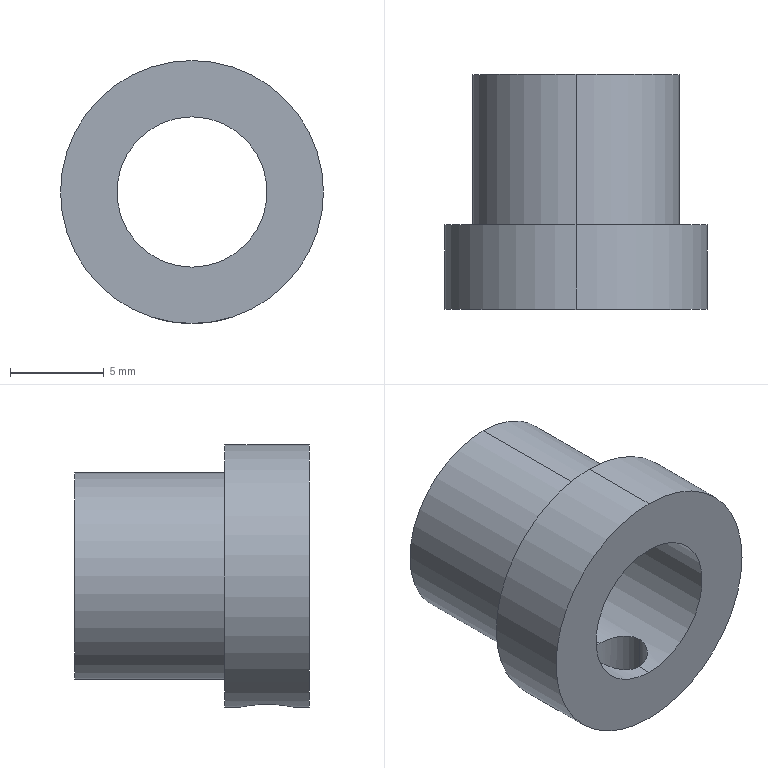Part | SolidWorks | features ICE 1, Revolution 1 | 1 solid | 11 faces | box 14 x 12.5 x 14 mm | volume 803.242 mm3 | cylinder 8 | plane 3 | commonest cylinder face diameters 3 x2 8 x2 11 x2 14 x2
STEP:
#1=CARTESIAN_POINT('',(0.,-4.489,-7.));
#2=VERTEX_POINT('',#1);
#3=CARTESIAN_POINT('',(-1.5,-2.989,-6.837));
#4=VERTEX_POINT('',#3);
#5=CARTESIAN_POINT('',(0.,-4.489,-7.));
#6=CARTESIAN_POINT('',(-0.1961,-4.489,-7.));
#7=CARTESIAN_POINT('',(-0.3941,-4.449,-6.991));
#8=CARTESIAN_POINT('',(-0.7554,-4.299,-6.961));
#9=CARTESIAN_POINT('',(-0.922,-4.188,-6.94));
#10=CARTESIAN_POINT('',(-1.13,-3.98,-6.909));
#11=CARTESIAN_POINT('',(-1.193,-3.904,-6.898));
#12=CARTESIAN_POINT('',(-1.301,-3.741,-6.878));
#13=CARTESIAN_POINT('',(-1.347,-3.655,-6.869));
#14=CARTESIAN_POINT('',(-1.461,-3.382,-6.846));
#15=CARTESIAN_POINT('',(-1.5,-3.187,-6.837));
#16=CARTESIAN_POINT('',(-1.5,-2.989,-6.837));
#17=B_SPLINE_CURVE_WITH_KNOTS('',3,(#5,#6,#7,#8,#9,#10,#11,#12,#13,#14,#15,#16),.UNSPECIFIED.,.F.,.F.,(4,2,2,2,2,4),(0.004703,0.005291,0.005879,0.006173,0.006467,0.007055),.UNSPECIFIED.);
#18=EDGE_CURVE('',#2,#4,#17,.T.);
#19=ORIENTED_EDGE('',*,*,#18,.T.);
#20=CARTESIAN_POINT('',(-1.5,-2.989,-3.708));
#21=VERTEX_POINT('',#20);
#22=CARTESIAN_POINT('',(-1.5,-2.989,-10.));
#23=DIRECTION('',(0.,0.,1.));
#24=VECTOR('',#23,1000.);
#25=LINE('',#22,#24);
#26=EDGE_CURVE('',#4,#21,#25,.T.);
#27=ORIENTED_EDGE('',*,*,#26,.T.);
#28=CARTESIAN_POINT('',(0.,-4.489,-4.));
#29=VERTEX_POINT('',#28);
#30=CARTESIAN_POINT('',(-1.5,-2.989,-3.708));
#31=CARTESIAN_POINT('',(-1.5,-3.087,-3.708));
#32=CARTESIAN_POINT('',(-1.49,-3.188,-3.712));
#33=CARTESIAN_POINT('',(-1.451,-3.381,-3.728));
#34=CARTESIAN_POINT('',(-1.422,-3.475,-3.739));
#35=CARTESIAN_POINT('',(-1.346,-3.658,-3.767));
#36=CARTESIAN_POINT('',(-1.3,-3.744,-3.783));
#37=CARTESIAN_POINT('',(-1.192,-3.905,-3.819));
#38=CARTESIAN_POINT('',(-1.129,-3.981,-3.838));
#39=CARTESIAN_POINT('',(-0.9911,-4.119,-3.876));
#40=CARTESIAN_POINT('',(-0.9163,-4.18,-3.895));
#41=CARTESIAN_POINT('',(-0.7543,-4.289,-3.929));
#42=CARTESIAN_POINT('',(-0.6667,-4.336,-3.945));
#43=CARTESIAN_POINT('',(-0.3961,-4.449,-3.985));
#44=CARTESIAN_POINT('',(-0.1971,-4.489,-4.));
#45=CARTESIAN_POINT('',(0.,-4.489,-4.));
#46=B_SPLINE_CURVE_WITH_KNOTS('',3,(#30,#31,#32,#33,#34,#35,#36,#37,#38,#39,#40,#41,#42,#43,#44,#45),.UNSPECIFIED.,.F.,.F.,(4,2,2,2,2,2,2,4),(0.002368,0.002663,0.002959,0.003255,0.00355,0.003846,0.004142,0.004733),.UNSPECIFIED.);
#47=EDGE_CURVE('',#21,#29,#46,.T.);
#48=ORIENTED_EDGE('',*,*,#47,.T.);
#49=CARTESIAN_POINT('',(1.5,-2.989,-3.708));
#50=VERTEX_POINT('',#49);
#51=CARTESIAN_POINT('',(0.,-4.489,-4.));
#52=CARTESIAN_POINT('',(0.1971,-4.489,-4.));
#53=CARTESIAN_POINT('',(0.3959,-4.449,-3.985));
#54=CARTESIAN_POINT('',(0.6677,-4.335,-3.945));
#55=CARTESIAN_POINT('',(0.7553,-4.288,-3.929));
#56=CARTESIAN_POINT('',(0.9168,-4.18,-3.894));
#57=CARTESIAN_POINT('',(0.9919,-4.118,-3.876));
#58=CARTESIAN_POINT('',(1.2,-3.91,-3.819));
#59=CARTESIAN_POINT('',(1.309,-3.747,-3.781));
#60=CARTESIAN_POINT('',(1.423,-3.474,-3.739));
#61=CARTESIAN_POINT('',(1.451,-3.381,-3.728));
#62=CARTESIAN_POINT('',(1.49,-3.188,-3.712));
#63=CARTESIAN_POINT('',(1.5,-3.087,-3.708));
#64=CARTESIAN_POINT('',(1.5,-2.989,-3.708));
#65=B_SPLINE_CURVE_WITH_KNOTS('',3,(#51,#52,#53,#54,#55,#56,#57,#58,#59,#60,#61,#62,#63,#64),.UNSPECIFIED.,.F.,.F.,(4,2,2,2,2,2,4),(0.004733,0.005325,0.00562,0.005916,0.006508,0.006803,0.007099),.UNSPECIFIED.);
#66=EDGE_CURVE('',#29,#50,#65,.T.);
#67=ORIENTED_EDGE('',*,*,#66,.T.);
#68=CARTESIAN_POINT('',(1.5,-2.989,-6.837));
#69=VERTEX_POINT('',#68);
#70=CARTESIAN_POINT('',(1.5,-2.989,-10.));
#71=DIRECTION('',(0.,0.,1.));
#72=VECTOR('',#71,1000.);
#73=LINE('',#70,#72);
#74=EDGE_CURVE('',#69,#50,#73,.T.);
#75=ORIENTED_EDGE('',*,*,#74,.F.);
#76=CARTESIAN_POINT('',(1.5,-2.989,-6.837));
#77=CARTESIAN_POINT('',(1.5,-3.087,-6.837));
#78=CARTESIAN_POINT('',(1.49,-3.186,-6.84));
#79=CARTESIAN_POINT('',(1.452,-3.379,-6.848));
#80=CARTESIAN_POINT('',(1.423,-3.473,-6.854));
#81=CARTESIAN_POINT('',(1.31,-3.745,-6.877));
#82=CARTESIAN_POINT('',(1.2,-3.91,-6.898));
#83=CARTESIAN_POINT('',(0.9907,-4.119,-6.93));
#84=CARTESIAN_POINT('',(0.9152,-4.181,-6.94));
#85=CARTESIAN_POINT('',(0.753,-4.29,-6.96));
#86=CARTESIAN_POINT('',(0.6652,-4.337,-6.969));
#87=CARTESIAN_POINT('',(0.484,-4.412,-6.984));
#88=CARTESIAN_POINT('',(0.3905,-4.44,-6.99));
#89=CARTESIAN_POINT('',(0.1976,-4.479,-6.998));
#90=CARTESIAN_POINT('',(0.09803,-4.489,-7.));
#91=CARTESIAN_POINT('',(0.,-4.489,-7.));
#92=B_SPLINE_CURVE_WITH_KNOTS('',3,(#76,#77,#78,#79,#80,#81,#82,#83,#84,#85,#86,#87,#88,#89,#90,#91),.UNSPECIFIED.,.F.,.F.,(4,2,2,2,2,2,2,4),(0.002352,0.002646,0.00294,0.003528,0.003822,0.004116,0.004409,0.004703),.UNSPECIFIED.);
#93=EDGE_CURVE('',#69,#2,#92,.T.);
#94=ORIENTED_EDGE('',*,*,#93,.T.);
#95=EDGE_LOOP('',(#19,#27,#48,#67,#75,#94));
#96=FACE_OUTER_BOUND('',#95,.T.);
#97=CARTESIAN_POINT('',(0.,-2.989,-10.));
#98=DIRECTION('',(0.,0.,1.));
#99=DIRECTION('',(1.,0.,0.));
#100=AXIS2_PLACEMENT_3D('',#97,#98,#99);
#101=CYLINDRICAL_SURFACE('',#100,1.5);
#102=ADVANCED_FACE('',(#96),#101,.F.);
#103=CARTESIAN_POINT('',(0.,-0.7386,-7.));
#104=VERTEX_POINT('',#103);
#105=CARTESIAN_POINT('',(0.,-0.7386,7.));
#106=VERTEX_POINT('',#105);
#107=CARTESIAN_POINT('',(0.,-0.7386,0.));
#108=DIRECTION('',(0.,-1.,0.));
#109=DIRECTION('',(0.,0.,-1.));
#110=AXIS2_PLACEMENT_3D('',#107,#108,#109);
#111=CIRCLE('',#110,7.);
#112=EDGE_CURVE('',#104,#106,#111,.T.);
#113=ORIENTED_EDGE('',*,*,#112,.T.);
#114=CARTESIAN_POINT('',(0.,-5.239,7.));
#115=VERTEX_POINT('',#114);
#116=CARTESIAN_POINT('',(0.,0.,7.));
#117=DIRECTION('',(0.,-1.,0.));
#118=VECTOR('',#117,1000.);
#119=LINE('',#116,#118);
#120=EDGE_CURVE('',#106,#115,#119,.T.);
#121=ORIENTED_EDGE('',*,*,#120,.T.);
#122=CARTESIAN_POINT('',(0.,-5.239,-7.));
#123=VERTEX_POINT('',#122);
#124=CARTESIAN_POINT('',(0.,-5.239,0.));
#125=DIRECTION('',(0.,-1.,0.));
#126=DIRECTION('',(0.,0.,-1.));
#127=AXIS2_PLACEMENT_3D('',#124,#125,#126);
#128=CIRCLE('',#127,7.);
#129=EDGE_CURVE('',#123,#115,#128,.T.);
#130=ORIENTED_EDGE('',*,*,#129,.F.);
#131=CARTESIAN_POINT('',(0.,0.,-7.));
#132=DIRECTION('',(0.,-1.,0.));
#133=VECTOR('',#132,1000.);
#134=LINE('',#131,#133);
#135=EDGE_CURVE('',#2,#123,#134,.T.);
#136=ORIENTED_EDGE('',*,*,#135,.F.);
#137=ORIENTED_EDGE('',*,*,#93,.F.);
#138=CARTESIAN_POINT('',(0.,-1.489,-7.));
#139=VERTEX_POINT('',#138);
#140=CARTESIAN_POINT('',(0.,-1.489,-7.));
#141=CARTESIAN_POINT('',(0.09944,-1.489,-7.));
#142=CARTESIAN_POINT('',(0.1972,-1.498,-6.998));
#143=CARTESIAN_POINT('',(0.3893,-1.537,-6.99));
#144=CARTESIAN_POINT('',(0.4848,-1.566,-6.984));
#145=CARTESIAN_POINT('',(0.6664,-1.641,-6.969));
#146=CARTESIAN_POINT('',(0.7524,-1.687,-6.96));
#147=CARTESIAN_POINT('',(0.9153,-1.796,-6.94));
#148=CARTESIAN_POINT('',(0.9922,-1.859,-6.93));
#149=CARTESIAN_POINT('',(1.199,-2.067,-6.898));
#150=CARTESIAN_POINT('',(1.311,-2.233,-6.877));
#151=CARTESIAN_POINT('',(1.46,-2.594,-6.846));
#152=CARTESIAN_POINT('',(1.5,-2.792,-6.837));
#153=CARTESIAN_POINT('',(1.5,-2.989,-6.837));
#154=B_SPLINE_CURVE_WITH_KNOTS('',3,(#140,#141,#142,#143,#144,#145,#146,#147,#148,#149,#150,#151,#152,#153),.UNSPECIFIED.,.F.,.F.,(4,2,2,2,2,2,4),(0.,0.000294,0.0005881,0.0008821,0.001176,0.001764,0.002352),.UNSPECIFIED.);
#155=EDGE_CURVE('',#139,#69,#154,.T.);
#156=ORIENTED_EDGE('',*,*,#155,.F.);
#157=CARTESIAN_POINT('',(0.,0.,-7.));
#158=DIRECTION('',(0.,-1.,0.));
#159=VECTOR('',#158,1000.);
#160=LINE('',#157,#159);
#161=EDGE_CURVE('',#104,#139,#160,.T.);
#162=ORIENTED_EDGE('',*,*,#161,.F.);
#163=EDGE_LOOP('',(#113,#121,#130,#136,#137,#156,#162));
#164=FACE_OUTER_BOUND('',#163,.T.);
#165=CARTESIAN_POINT('',(0.,0.,0.));
#166=DIRECTION('',(0.,-1.,0.));
#167=DIRECTION('',(0.,0.,-1.));
#168=AXIS2_PLACEMENT_3D('',#165,#166,#167);
#169=CYLINDRICAL_SURFACE('',#168,7.);
#170=ADVANCED_FACE('',(#164),#169,.T.);
#171=CARTESIAN_POINT('',(0.,7.261,-5.5));
#172=VERTEX_POINT('',#171);
#173=CARTESIAN_POINT('',(0.,7.261,5.5));
#174=VERTEX_POINT('',#173);
#175=CARTESIAN_POINT('',(0.,7.261,0.));
#176=DIRECTION('',(0.,-1.,0.));
#177=DIRECTION('',(0.,0.,-1.));
#178=AXIS2_PLACEMENT_3D('',#175,#176,#177);
#179=CIRCLE('',#178,5.5);
#180=EDGE_CURVE('',#172,#174,#179,.T.);
#181=ORIENTED_EDGE('',*,*,#180,.T.);
#182=CARTESIAN_POINT('',(0.,-0.7386,5.5));
#183=VERTEX_POINT('',#182);
#184=CARTESIAN_POINT('',(0.,0.,5.5));
#185=DIRECTION('',(0.,-1.,0.));
#186=VECTOR('',#185,1000.);
#187=LINE('',#184,#186);
#188=EDGE_CURVE('',#174,#183,#187,.T.);
#189=ORIENTED_EDGE('',*,*,#188,.T.);
#190=CARTESIAN_POINT('',(0.,-0.7386,-5.5));
#191=VERTEX_POINT('',#190);
#192=CARTESIAN_POINT('',(0.,-0.7386,0.));
#193=DIRECTION('',(0.,-1.,0.));
#194=DIRECTION('',(0.,0.,-1.));
#195=AXIS2_PLACEMENT_3D('',#192,#193,#194);
#196=CIRCLE('',#195,5.5);
#197=EDGE_CURVE('',#191,#183,#196,.T.);
#198=ORIENTED_EDGE('',*,*,#197,.F.);
#199=CARTESIAN_POINT('',(0.,0.,-5.5));
#200=DIRECTION('',(0.,-1.,0.));
#201=VECTOR('',#200,1000.);
#202=LINE('',#199,#201);
#203=EDGE_CURVE('',#172,#191,#202,.T.);
#204=ORIENTED_EDGE('',*,*,#203,.F.);
#205=EDGE_LOOP('',(#181,#189,#198,#204));
#206=FACE_OUTER_BOUND('',#205,.T.);
#207=CARTESIAN_POINT('',(0.,0.,0.));
#208=DIRECTION('',(0.,-1.,0.));
#209=DIRECTION('',(0.,0.,-1.));
#210=AXIS2_PLACEMENT_3D('',#207,#208,#209);
#211=CYLINDRICAL_SURFACE('',#210,5.5);
#212=ADVANCED_FACE('',(#206),#211,.T.);
#213=CARTESIAN_POINT('',(0.,7.261,4.));
#214=VERTEX_POINT('',#213);
#215=CARTESIAN_POINT('',(0.,7.261,-4.));
#216=VERTEX_POINT('',#215);
#217=CARTESIAN_POINT('',(0.,7.261,0.));
#218=DIRECTION('',(0.,-1.,0.));
#219=DIRECTION('',(0.,0.,-1.));
#220=AXIS2_PLACEMENT_3D('',#217,#218,#219);
#221=CIRCLE('',#220,4.);
#222=EDGE_CURVE('',#214,#216,#221,.T.);
#223=ORIENTED_EDGE('',*,*,#222,.F.);
#224=CARTESIAN_POINT('',(0.,-5.239,4.));
#225=VERTEX_POINT('',#224);
#226=CARTESIAN_POINT('',(0.,0.,4.));
#227=DIRECTION('',(0.,-1.,0.));
#228=VECTOR('',#227,1000.);
#229=LINE('',#226,#228);
#230=EDGE_CURVE('',#214,#225,#229,.T.);
#231=ORIENTED_EDGE('',*,*,#230,.T.);
#232=CARTESIAN_POINT('',(0.,-5.239,-4.));
#233=VERTEX_POINT('',#232);
#234=CARTESIAN_POINT('',(0.,-5.239,0.));
#235=DIRECTION('',(0.,-1.,0.));
#236=DIRECTION('',(0.,0.,-1.));
#237=AXIS2_PLACEMENT_3D('',#234,#235,#236);
#238=CIRCLE('',#237,4.);
#239=EDGE_CURVE('',#225,#233,#238,.T.);
#240=ORIENTED_EDGE('',*,*,#239,.T.);
#241=CARTESIAN_POINT('',(0.,0.,-4.));
#242=DIRECTION('',(0.,-1.,0.));
#243=VECTOR('',#242,1000.);
#244=LINE('',#241,#243);
#245=EDGE_CURVE('',#29,#233,#244,.T.);
#246=ORIENTED_EDGE('',*,*,#245,.F.);
#247=ORIENTED_EDGE('',*,*,#47,.F.);
#248=CARTESIAN_POINT('',(0.,-1.489,-4.));
#249=VERTEX_POINT('',#248);
#250=CARTESIAN_POINT('',(0.,-1.489,-4.));
#251=CARTESIAN_POINT('',(-0.1001,-1.489,-4.));
#252=CARTESIAN_POINT('',(-0.1984,-1.499,-3.996));
#253=CARTESIAN_POINT('',(-0.3915,-1.537,-3.982));
#254=CARTESIAN_POINT('',(-0.4873,-1.567,-3.971));
#255=CARTESIAN_POINT('',(-0.7594,-1.68,-3.932));
#256=CARTESIAN_POINT('',(-0.9246,-1.792,-3.894));
#257=CARTESIAN_POINT('',(-1.199,-2.066,-3.819));
#258=CARTESIAN_POINT('',(-1.31,-2.232,-3.78));
#259=CARTESIAN_POINT('',(-1.422,-2.502,-3.739));
#260=CARTESIAN_POINT('',(-1.452,-2.598,-3.727));
#261=CARTESIAN_POINT('',(-1.49,-2.792,-3.712));
#262=CARTESIAN_POINT('',(-1.5,-2.89,-3.708));
#263=CARTESIAN_POINT('',(-1.5,-2.989,-3.708));
#264=B_SPLINE_CURVE_WITH_KNOTS('',3,(#250,#251,#252,#253,#254,#255,#256,#257,#258,#259,#260,#261,#262,#263),.UNSPECIFIED.,.F.,.F.,(4,2,2,2,2,2,4),(0.,0.0002959,0.0005919,0.001184,0.001776,0.002072,0.002368),.UNSPECIFIED.);
#265=EDGE_CURVE('',#249,#21,#264,.T.);
#266=ORIENTED_EDGE('',*,*,#265,.F.);
#267=CARTESIAN_POINT('',(0.,0.,-4.));
#268=DIRECTION('',(0.,-1.,0.));
#269=VECTOR('',#268,1000.);
#270=LINE('',#267,#269);
#271=EDGE_CURVE('',#216,#249,#270,.T.);
#272=ORIENTED_EDGE('',*,*,#271,.F.);
#273=EDGE_LOOP('',(#223,#231,#240,#246,#247,#266,#272));
#274=FACE_OUTER_BOUND('',#273,.T.);
#275=CARTESIAN_POINT('',(0.,0.,0.));
#276=DIRECTION('',(0.,-1.,0.));
#277=DIRECTION('',(0.,0.,-1.));
#278=AXIS2_PLACEMENT_3D('',#275,#276,#277);
#279=CYLINDRICAL_SURFACE('',#278,4.);
#280=ADVANCED_FACE('',(#274),#279,.F.);
#281=ORIENTED_EDGE('',*,*,#230,.F.);
#282=CARTESIAN_POINT('',(0.,7.261,0.));
#283=DIRECTION('',(0.,-1.,0.));
#284=DIRECTION('',(0.,0.,-1.));
#285=AXIS2_PLACEMENT_3D('',#282,#283,#284);
#286=CIRCLE('',#285,4.);
#287=EDGE_CURVE('',#216,#214,#286,.T.);
#288=ORIENTED_EDGE('',*,*,#287,.F.);
#289=ORIENTED_EDGE('',*,*,#271,.T.);
#290=CARTESIAN_POINT('',(1.5,-2.989,-3.708));
#291=CARTESIAN_POINT('',(1.5,-2.791,-3.708));
#292=CARTESIAN_POINT('',(1.46,-2.592,-3.725));
#293=CARTESIAN_POINT('',(1.309,-2.231,-3.781));
#294=CARTESIAN_POINT('',(1.198,-2.065,-3.819));
#295=CARTESIAN_POINT('',(0.9918,-1.859,-3.876));
#296=CARTESIAN_POINT('',(0.9153,-1.796,-3.895));
#297=CARTESIAN_POINT('',(0.7537,-1.688,-3.929));
#298=CARTESIAN_POINT('',(0.6679,-1.642,-3.945));
#299=CARTESIAN_POINT('',(0.3946,-1.528,-3.985));
#300=CARTESIAN_POINT('',(0.2002,-1.489,-4.));
#301=CARTESIAN_POINT('',(0.,-1.489,-4.));
#302=B_SPLINE_CURVE_WITH_KNOTS('',3,(#290,#291,#292,#293,#294,#295,#296,#297,#298,#299,#300,#301),.UNSPECIFIED.,.F.,.F.,(4,2,2,2,2,4),(0.007099,0.007691,0.008282,0.008578,0.008874,0.009466),.UNSPECIFIED.);
#303=EDGE_CURVE('',#50,#249,#302,.T.);
#304=ORIENTED_EDGE('',*,*,#303,.F.);
#305=ORIENTED_EDGE('',*,*,#66,.F.);
#306=ORIENTED_EDGE('',*,*,#245,.T.);
#307=CARTESIAN_POINT('',(0.,-5.239,0.));
#308=DIRECTION('',(0.,-1.,0.));
#309=DIRECTION('',(0.,0.,-1.));
#310=AXIS2_PLACEMENT_3D('',#307,#308,#309);
#311=CIRCLE('',#310,4.);
#312=EDGE_CURVE('',#233,#225,#311,.T.);
#313=ORIENTED_EDGE('',*,*,#312,.T.);
#314=EDGE_LOOP('',(#281,#288,#289,#304,#305,#306,#313));
#315=FACE_OUTER_BOUND('',#314,.T.);
#316=CARTESIAN_POINT('',(0.,0.,0.));
#317=DIRECTION('',(0.,-1.,0.));
#318=DIRECTION('',(0.,0.,-1.));
#319=AXIS2_PLACEMENT_3D('',#316,#317,#318);
#320=CYLINDRICAL_SURFACE('',#319,4.);
#321=ADVANCED_FACE('',(#315),#320,.F.);
#322=ORIENTED_EDGE('',*,*,#287,.T.);
#323=ORIENTED_EDGE('',*,*,#222,.T.);
#324=EDGE_LOOP('',(#322,#323));
#325=FACE_BOUND('',#324,.T.);
#326=ORIENTED_EDGE('',*,*,#180,.F.);
#327=CARTESIAN_POINT('',(0.,7.261,0.));
#328=DIRECTION('',(0.,-1.,0.));
#329=DIRECTION('',(0.,0.,-1.));
#330=AXIS2_PLACEMENT_3D('',#327,#328,#329);
#331=CIRCLE('',#330,5.5);
#332=EDGE_CURVE('',#174,#172,#331,.T.);
#333=ORIENTED_EDGE('',*,*,#332,.F.);
#334=EDGE_LOOP('',(#326,#333));
#335=FACE_OUTER_BOUND('',#334,.T.);
#336=CARTESIAN_POINT('',(4.,7.261,0.));
#337=DIRECTION('',(0.,1.,0.));
#338=DIRECTION('',(0.,0.,1.));
#339=AXIS2_PLACEMENT_3D('',#336,#337,#338);
#340=PLANE('',#339);
#341=ADVANCED_FACE('',(#325,#335),#340,.T.);
#342=ORIENTED_EDGE('',*,*,#188,.F.);
#343=ORIENTED_EDGE('',*,*,#332,.T.);
#344=ORIENTED_EDGE('',*,*,#203,.T.);
#345=CARTESIAN_POINT('',(0.,-0.7386,0.));
#346=DIRECTION('',(0.,-1.,0.));
#347=DIRECTION('',(0.,0.,-1.));
#348=AXIS2_PLACEMENT_3D('',#345,#346,#347);
#349=CIRCLE('',#348,5.5);
#350=EDGE_CURVE('',#183,#191,#349,.T.);
#351=ORIENTED_EDGE('',*,*,#350,.F.);
#352=EDGE_LOOP('',(#342,#343,#344,#351));
#353=FACE_OUTER_BOUND('',#352,.T.);
#354=CARTESIAN_POINT('',(0.,0.,0.));
#355=DIRECTION('',(0.,-1.,0.));
#356=DIRECTION('',(0.,0.,-1.));
#357=AXIS2_PLACEMENT_3D('',#354,#355,#356);
#358=CYLINDRICAL_SURFACE('',#357,5.5);
#359=ADVANCED_FACE('',(#353),#358,.T.);
#360=ORIENTED_EDGE('',*,*,#197,.T.);
#361=ORIENTED_EDGE('',*,*,#350,.T.);
#362=EDGE_LOOP('',(#360,#361));
#363=FACE_BOUND('',#362,.T.);
#364=ORIENTED_EDGE('',*,*,#112,.F.);
#365=CARTESIAN_POINT('',(0.,-0.7386,0.));
#366=DIRECTION('',(0.,-1.,0.));
#367=DIRECTION('',(0.,0.,-1.));
#368=AXIS2_PLACEMENT_3D('',#365,#366,#367);
#369=CIRCLE('',#368,7.);
#370=EDGE_CURVE('',#106,#104,#369,.T.);
#371=ORIENTED_EDGE('',*,*,#370,.F.);
#372=EDGE_LOOP('',(#364,#371));
#373=FACE_OUTER_BOUND('',#372,.T.);
#374=CARTESIAN_POINT('',(5.5,-0.7386,0.));
#375=DIRECTION('',(0.,1.,0.));
#376=DIRECTION('',(0.,0.,1.));
#377=AXIS2_PLACEMENT_3D('',#374,#375,#376);
#378=PLANE('',#377);
#379=ADVANCED_FACE('',(#363,#373),#378,.T.);
#380=ORIENTED_EDGE('',*,*,#120,.F.);
#381=ORIENTED_EDGE('',*,*,#370,.T.);
#382=ORIENTED_EDGE('',*,*,#161,.T.);
#383=CARTESIAN_POINT('',(-1.5,-2.989,-6.837));
#384=CARTESIAN_POINT('',(-1.5,-2.89,-6.837));
#385=CARTESIAN_POINT('',(-1.49,-2.792,-6.84));
#386=CARTESIAN_POINT('',(-1.452,-2.6,-6.848));
#387=CARTESIAN_POINT('',(-1.423,-2.504,-6.854));
#388=CARTESIAN_POINT('',(-1.31,-2.233,-6.877));
#389=CARTESIAN_POINT('',(-1.199,-2.066,-6.898));
#390=CARTESIAN_POINT('',(-0.9234,-1.791,-6.94));
#391=CARTESIAN_POINT('',(-0.7567,-1.679,-6.961));
#392=CARTESIAN_POINT('',(-0.3959,-1.529,-6.991));
#393=CARTESIAN_POINT('',(-0.1987,-1.489,-7.));
#394=CARTESIAN_POINT('',(0.,-1.489,-7.));
#395=B_SPLINE_CURVE_WITH_KNOTS('',3,(#383,#384,#385,#386,#387,#388,#389,#390,#391,#392,#393,#394),.UNSPECIFIED.,.F.,.F.,(4,2,2,2,2,4),(0.007055,0.007349,0.007643,0.00823,0.008818,0.009405),.UNSPECIFIED.);
#396=EDGE_CURVE('',#4,#139,#395,.T.);
#397=ORIENTED_EDGE('',*,*,#396,.F.);
#398=ORIENTED_EDGE('',*,*,#18,.F.);
#399=ORIENTED_EDGE('',*,*,#135,.T.);
#400=CARTESIAN_POINT('',(0.,-5.239,0.));
#401=DIRECTION('',(0.,-1.,0.));
#402=DIRECTION('',(0.,0.,-1.));
#403=AXIS2_PLACEMENT_3D('',#400,#401,#402);
#404=CIRCLE('',#403,7.);
#405=EDGE_CURVE('',#115,#123,#404,.T.);
#406=ORIENTED_EDGE('',*,*,#405,.F.);
#407=EDGE_LOOP('',(#380,#381,#382,#397,#398,#399,#406));
#408=FACE_OUTER_BOUND('',#407,.T.);
#409=CARTESIAN_POINT('',(0.,0.,0.));
#410=DIRECTION('',(0.,-1.,0.));
#411=DIRECTION('',(0.,0.,-1.));
#412=AXIS2_PLACEMENT_3D('',#409,#410,#411);
#413=CYLINDRICAL_SURFACE('',#412,7.);
#414=ADVANCED_FACE('',(#408),#413,.T.);
#415=ORIENTED_EDGE('',*,*,#129,.T.);
#416=ORIENTED_EDGE('',*,*,#405,.T.);
#417=EDGE_LOOP('',(#415,#416));
#418=FACE_OUTER_BOUND('',#417,.T.);
#419=ORIENTED_EDGE('',*,*,#312,.F.);
#420=ORIENTED_EDGE('',*,*,#239,.F.);
#421=EDGE_LOOP('',(#419,#420));
#422=FACE_BOUND('',#421,.T.);
#423=CARTESIAN_POINT('',(7.,-5.239,0.));
#424=DIRECTION('',(0.,-1.,0.));
#425=DIRECTION('',(0.,0.,-1.));
#426=AXIS2_PLACEMENT_3D('',#423,#424,#425);
#427=PLANE('',#426);
#428=ADVANCED_FACE('',(#418,#422),#427,.T.);
#429=ORIENTED_EDGE('',*,*,#26,.F.);
#430=ORIENTED_EDGE('',*,*,#396,.T.);
#431=ORIENTED_EDGE('',*,*,#155,.T.);
#432=ORIENTED_EDGE('',*,*,#74,.T.);
#433=ORIENTED_EDGE('',*,*,#303,.T.);
#434=ORIENTED_EDGE('',*,*,#265,.T.);
#435=EDGE_LOOP('',(#429,#430,#431,#432,#433,#434));
#436=FACE_OUTER_BOUND('',#435,.T.);
#437=CARTESIAN_POINT('',(0.,-2.989,-10.));
#438=DIRECTION('',(0.,0.,1.));
#439=DIRECTION('',(1.,0.,0.));
#440=AXIS2_PLACEMENT_3D('',#437,#438,#439);
#441=CYLINDRICAL_SURFACE('',#440,1.5);
#442=ADVANCED_FACE('',(#436),#441,.F.);
#443=CLOSED_SHELL('',(#102,#170,#212,#280,#321,#341,#359,#379,#414,#428,#442));
#444=MANIFOLD_SOLID_BREP('',#443);
#445=CARTESIAN_POINT('',(0.,0.,0.));
#446=DIRECTION('',(0.,0.,1.));
#447=DIRECTION('',(1.,0.,0.));
#448=AXIS2_PLACEMENT_3D('',#445,#446,#447);
#449=(LENGTH_UNIT()NAMED_UNIT(*)SI_UNIT(.MILLI.,.METRE.));
#450=UNCERTAINTY_MEASURE_WITH_UNIT(LENGTH_MEASURE(0.00001),#449,'','');
#451=(NAMED_UNIT(*)PLANE_ANGLE_UNIT()SI_UNIT($,.RADIAN.));
#452=(NAMED_UNIT(*)SI_UNIT($,.STERADIAN.)SOLID_ANGLE_UNIT());
#453=(GEOMETRIC_REPRESENTATION_CONTEXT(3)GLOBAL_UNCERTAINTY_ASSIGNED_CONTEXT((#450))GLOBAL_UNIT_ASSIGNED_CONTEXT((#449,#451,#452))REPRESENTATION_CONTEXT('',''));
#454=ADVANCED_BREP_SHAPE_REPRESENTATION('',(#444,#448),#453);